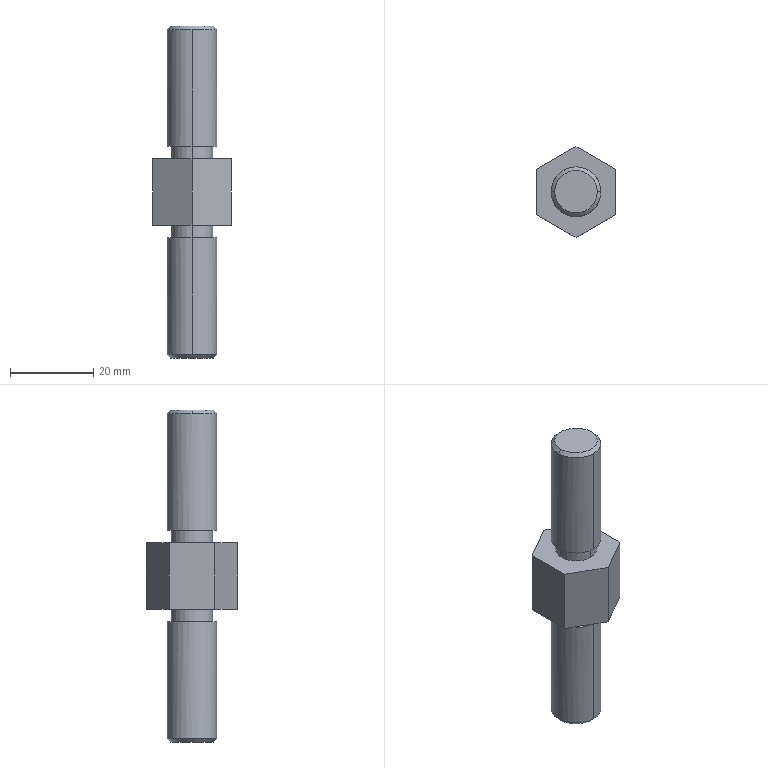Part | NX | 1 solid | 24 faces | box 19 x 21.939 x 80 mm | volume 12006 mm3 | plane 12 | cylinder 8 | cone 4 | commonest cylinder face diameters 10 x4 12 x4
STEP:
#1=CARTESIAN_POINT('',(0.,6.,11.));
#2=VERTEX_POINT('',#1);
#3=CARTESIAN_POINT('',(0.,-6.,11.));
#4=VERTEX_POINT('',#3);
#5=CARTESIAN_POINT('',(0.,0.,11.));
#6=DIRECTION('',(0.,0.,1.));
#7=DIRECTION('',(0.,-1.,0.));
#8=AXIS2_PLACEMENT_3D('',#5,#6,#7);
#9=CIRCLE('',#8,6.);
#10=EDGE_CURVE('',#2,#4,#9,.T.);
#11=ORIENTED_EDGE('',*,*,#10,.T.);
#12=CARTESIAN_POINT('',(0.,-6.,39.125));
#13=VERTEX_POINT('',#12);
#14=CARTESIAN_POINT('',(0.,-6.,5.));
#15=DIRECTION('',(0.,0.,1.));
#16=VECTOR('',#15,1000.);
#17=LINE('',#14,#16);
#18=EDGE_CURVE('',#13,#4,#17,.F.);
#19=ORIENTED_EDGE('',*,*,#18,.F.);
#20=CARTESIAN_POINT('',(-6.,0.,39.125));
#21=VERTEX_POINT('',#20);
#22=CARTESIAN_POINT('',(0.,0.,39.125));
#23=DIRECTION('',(0.,0.,-1.));
#24=DIRECTION('',(-1.,0.,0.));
#25=AXIS2_PLACEMENT_3D('',#22,#23,#24);
#26=CIRCLE('',#25,6.);
#27=EDGE_CURVE('',#13,#21,#26,.T.);
#28=ORIENTED_EDGE('',*,*,#27,.T.);
#29=CARTESIAN_POINT('',(0.,6.,39.125));
#30=VERTEX_POINT('',#29);
#31=CARTESIAN_POINT('',(0.,0.,39.125));
#32=DIRECTION('',(0.,0.,-1.));
#33=DIRECTION('',(-1.,0.,0.));
#34=AXIS2_PLACEMENT_3D('',#31,#32,#33);
#35=CIRCLE('',#34,6.);
#36=EDGE_CURVE('',#21,#30,#35,.T.);
#37=ORIENTED_EDGE('',*,*,#36,.T.);
#38=CARTESIAN_POINT('',(0.,6.,5.));
#39=DIRECTION('',(0.,0.,1.));
#40=VECTOR('',#39,1000.);
#41=LINE('',#38,#40);
#42=EDGE_CURVE('',#30,#2,#41,.F.);
#43=ORIENTED_EDGE('',*,*,#42,.T.);
#44=EDGE_LOOP('',(#11,#19,#28,#37,#43));
#45=FACE_BOUND('',#44,.T.);
#46=CARTESIAN_POINT('',(0.,0.,5.));
#47=DIRECTION('',(0.,0.,1.));
#48=DIRECTION('',(0.,-1.,0.));
#49=AXIS2_PLACEMENT_3D('',#46,#47,#48);
#50=CYLINDRICAL_SURFACE('',#49,6.);
#51=ADVANCED_FACE('',(#45),#50,.T.);
#52=CARTESIAN_POINT('',(5.125,0.,40.));
#53=VERTEX_POINT('',#52);
#54=CARTESIAN_POINT('',(-5.125,0.,40.));
#55=VERTEX_POINT('',#54);
#56=CARTESIAN_POINT('',(0.,0.,40.));
#57=DIRECTION('',(0.,0.,-1.));
#58=DIRECTION('',(-1.,0.,0.));
#59=AXIS2_PLACEMENT_3D('',#56,#57,#58);
#60=CIRCLE('',#59,5.125);
#61=EDGE_CURVE('',#53,#55,#60,.T.);
#62=ORIENTED_EDGE('',*,*,#61,.F.);
#63=CARTESIAN_POINT('',(0.,0.,40.));
#64=DIRECTION('',(0.,0.,-1.));
#65=DIRECTION('',(-1.,0.,0.));
#66=AXIS2_PLACEMENT_3D('',#63,#64,#65);
#67=CIRCLE('',#66,5.125);
#68=EDGE_CURVE('',#55,#53,#67,.T.);
#69=ORIENTED_EDGE('',*,*,#68,.F.);
#70=EDGE_LOOP('',(#62,#69));
#71=FACE_BOUND('',#70,.T.);
#72=CARTESIAN_POINT('',(-4.214,5.931,40.));
#73=DIRECTION('',(0.,0.,1.));
#74=DIRECTION('',(1.,0.,0.));
#75=AXIS2_PLACEMENT_3D('',#72,#73,#74);
#76=PLANE('',#75);
#77=ADVANCED_FACE('',(#71),#76,.T.);
#78=CARTESIAN_POINT('',(0.,6.,-11.));
#79=VERTEX_POINT('',#78);
#80=CARTESIAN_POINT('',(0.,-6.,-11.));
#81=VERTEX_POINT('',#80);
#82=CARTESIAN_POINT('',(0.,0.,-11.));
#83=DIRECTION('',(0.,0.,-1.));
#84=DIRECTION('',(0.,-1.,0.));
#85=AXIS2_PLACEMENT_3D('',#82,#83,#84);
#86=CIRCLE('',#85,6.);
#87=EDGE_CURVE('',#79,#81,#86,.T.);
#88=ORIENTED_EDGE('',*,*,#87,.F.);
#89=CARTESIAN_POINT('',(0.,0.,-11.));
#90=DIRECTION('',(0.,0.,-1.));
#91=DIRECTION('',(0.,-1.,0.));
#92=AXIS2_PLACEMENT_3D('',#89,#90,#91);
#93=CIRCLE('',#92,6.);
#94=EDGE_CURVE('',#81,#79,#93,.T.);
#95=ORIENTED_EDGE('',*,*,#94,.F.);
#96=EDGE_LOOP('',(#88,#95));
#97=FACE_BOUND('',#96,.T.);
#98=CARTESIAN_POINT('',(0.,-5.,-11.));
#99=VERTEX_POINT('',#98);
#100=CARTESIAN_POINT('',(0.,5.,-11.));
#101=VERTEX_POINT('',#100);
#102=CARTESIAN_POINT('',(0.,0.,-11.));
#103=DIRECTION('',(0.,0.,-1.));
#104=DIRECTION('',(0.,1.,0.));
#105=AXIS2_PLACEMENT_3D('',#102,#103,#104);
#106=CIRCLE('',#105,5.);
#107=EDGE_CURVE('',#99,#101,#106,.T.);
#108=ORIENTED_EDGE('',*,*,#107,.T.);
#109=CARTESIAN_POINT('',(0.,0.,-11.));
#110=DIRECTION('',(0.,0.,-1.));
#111=DIRECTION('',(0.,1.,0.));
#112=AXIS2_PLACEMENT_3D('',#109,#110,#111);
#113=CIRCLE('',#112,5.);
#114=EDGE_CURVE('',#101,#99,#113,.T.);
#115=ORIENTED_EDGE('',*,*,#114,.T.);
#116=EDGE_LOOP('',(#108,#115));
#117=FACE_BOUND('',#116,.T.);
#118=CARTESIAN_POINT('',(-2.472,7.007,-11.));
#119=DIRECTION('',(0.,0.,-1.));
#120=DIRECTION('',(0.,-1.,0.));
#121=AXIS2_PLACEMENT_3D('',#118,#119,#120);
#122=PLANE('',#121);
#123=ADVANCED_FACE('',(#97,#117),#122,.F.);
#124=CARTESIAN_POINT('',(-9.5,5.485,8.));
#125=VERTEX_POINT('',#124);
#126=CARTESIAN_POINT('',(-9.5,5.485,-8.));
#127=VERTEX_POINT('',#126);
#128=CARTESIAN_POINT('',(-9.5,5.485,0.));
#129=DIRECTION('',(0.,0.,-1.));
#130=VECTOR('',#129,1000.);
#131=LINE('',#128,#130);
#132=EDGE_CURVE('',#125,#127,#131,.T.);
#133=ORIENTED_EDGE('',*,*,#132,.F.);
#134=CARTESIAN_POINT('',(0.,10.97,8.));
#135=VERTEX_POINT('',#134);
#136=CARTESIAN_POINT('',(0.,10.97,8.));
#137=DIRECTION('',(0.866,0.5,0.));
#138=VECTOR('',#137,1000.);
#139=LINE('',#136,#138);
#140=EDGE_CURVE('',#125,#135,#139,.T.);
#141=ORIENTED_EDGE('',*,*,#140,.T.);
#142=CARTESIAN_POINT('',(0.,10.97,-8.));
#143=VERTEX_POINT('',#142);
#144=CARTESIAN_POINT('',(0.,10.97,0.));
#145=DIRECTION('',(0.,0.,1.));
#146=VECTOR('',#145,1000.);
#147=LINE('',#144,#146);
#148=EDGE_CURVE('',#143,#135,#147,.T.);
#149=ORIENTED_EDGE('',*,*,#148,.F.);
#150=CARTESIAN_POINT('',(0.,10.97,-8.));
#151=DIRECTION('',(0.866,0.5,0.));
#152=VECTOR('',#151,1000.);
#153=LINE('',#150,#152);
#154=EDGE_CURVE('',#127,#143,#153,.T.);
#155=ORIENTED_EDGE('',*,*,#154,.F.);
#156=EDGE_LOOP('',(#133,#141,#149,#155));
#157=FACE_BOUND('',#156,.T.);
#158=CARTESIAN_POINT('',(-9.5,5.485,0.));
#159=DIRECTION('',(-0.5,0.866,0.));
#160=DIRECTION('',(0.,0.,1.));
#161=AXIS2_PLACEMENT_3D('',#158,#159,#160);
#162=PLANE('',#161);
#163=ADVANCED_FACE('',(#157),#162,.T.);
#164=CARTESIAN_POINT('',(9.5,5.485,8.));
#165=VERTEX_POINT('',#164);
#166=CARTESIAN_POINT('',(9.5,-5.485,8.));
#167=VERTEX_POINT('',#166);
#168=CARTESIAN_POINT('',(9.5,0.,8.));
#169=DIRECTION('',(0.,-1.,0.));
#170=VECTOR('',#169,1000.);
#171=LINE('',#168,#170);
#172=EDGE_CURVE('',#165,#167,#171,.T.);
#173=ORIENTED_EDGE('',*,*,#172,.F.);
#174=CARTESIAN_POINT('',(0.,10.97,8.));
#175=DIRECTION('',(0.866,-0.5,0.));
#176=VECTOR('',#175,1000.);
#177=LINE('',#174,#176);
#178=EDGE_CURVE('',#135,#165,#177,.T.);
#179=ORIENTED_EDGE('',*,*,#178,.F.);
#180=ORIENTED_EDGE('',*,*,#140,.F.);
#181=CARTESIAN_POINT('',(-9.5,-5.485,8.));
#182=VERTEX_POINT('',#181);
#183=CARTESIAN_POINT('',(-9.5,0.,8.));
#184=DIRECTION('',(0.,1.,0.));
#185=VECTOR('',#184,1000.);
#186=LINE('',#183,#185);
#187=EDGE_CURVE('',#182,#125,#186,.T.);
#188=ORIENTED_EDGE('',*,*,#187,.F.);
#189=CARTESIAN_POINT('',(0.,-10.97,8.));
#190=VERTEX_POINT('',#189);
#191=CARTESIAN_POINT('',(0.,-10.97,8.));
#192=DIRECTION('',(-0.866,0.5,0.));
#193=VECTOR('',#192,1000.);
#194=LINE('',#191,#193);
#195=EDGE_CURVE('',#190,#182,#194,.T.);
#196=ORIENTED_EDGE('',*,*,#195,.F.);
#197=CARTESIAN_POINT('',(0.,-10.97,8.));
#198=DIRECTION('',(-0.866,-0.5,0.));
#199=VECTOR('',#198,1000.);
#200=LINE('',#197,#199);
#201=EDGE_CURVE('',#167,#190,#200,.T.);
#202=ORIENTED_EDGE('',*,*,#201,.F.);
#203=EDGE_LOOP('',(#173,#179,#180,#188,#196,#202));
#204=FACE_BOUND('',#203,.T.);
#205=CARTESIAN_POINT('',(0.,-5.,8.));
#206=VERTEX_POINT('',#205);
#207=CARTESIAN_POINT('',(0.,5.,8.));
#208=VERTEX_POINT('',#207);
#209=CARTESIAN_POINT('',(0.,0.,8.));
#210=DIRECTION('',(0.,0.,-1.));
#211=DIRECTION('',(0.,1.,0.));
#212=AXIS2_PLACEMENT_3D('',#209,#210,#211);
#213=CIRCLE('',#212,5.);
#214=EDGE_CURVE('',#206,#208,#213,.T.);
#215=ORIENTED_EDGE('',*,*,#214,.T.);
#216=CARTESIAN_POINT('',(0.,0.,8.));
#217=DIRECTION('',(0.,0.,-1.));
#218=DIRECTION('',(0.,1.,0.));
#219=AXIS2_PLACEMENT_3D('',#216,#217,#218);
#220=CIRCLE('',#219,5.);
#221=EDGE_CURVE('',#208,#206,#220,.T.);
#222=ORIENTED_EDGE('',*,*,#221,.T.);
#223=EDGE_LOOP('',(#215,#222));
#224=FACE_BOUND('',#223,.T.);
#225=CARTESIAN_POINT('',(-2.472,7.007,8.));
#226=DIRECTION('',(0.,0.,-1.));
#227=DIRECTION('',(0.,-1.,0.));
#228=AXIS2_PLACEMENT_3D('',#225,#226,#227);
#229=PLANE('',#228);
#230=ADVANCED_FACE('',(#204,#224),#229,.F.);
#231=CARTESIAN_POINT('',(9.5,-5.485,-8.));
#232=VERTEX_POINT('',#231);
#233=CARTESIAN_POINT('',(0.,-10.97,-8.));
#234=VERTEX_POINT('',#233);
#235=CARTESIAN_POINT('',(0.,-10.97,-8.));
#236=DIRECTION('',(-0.866,-0.5,0.));
#237=VECTOR('',#236,1000.);
#238=LINE('',#235,#237);
#239=EDGE_CURVE('',#232,#234,#238,.T.);
#240=ORIENTED_EDGE('',*,*,#239,.F.);
#241=CARTESIAN_POINT('',(9.5,-5.485,0.));
#242=DIRECTION('',(0.,0.,-1.));
#243=VECTOR('',#242,1000.);
#244=LINE('',#241,#243);
#245=EDGE_CURVE('',#167,#232,#244,.T.);
#246=ORIENTED_EDGE('',*,*,#245,.F.);
#247=ORIENTED_EDGE('',*,*,#201,.T.);
#248=CARTESIAN_POINT('',(0.,-10.97,0.));
#249=DIRECTION('',(0.,0.,-1.));
#250=VECTOR('',#249,1000.);
#251=LINE('',#248,#250);
#252=EDGE_CURVE('',#190,#234,#251,.T.);
#253=ORIENTED_EDGE('',*,*,#252,.T.);
#254=EDGE_LOOP('',(#240,#246,#247,#253));
#255=FACE_BOUND('',#254,.T.);
#256=CARTESIAN_POINT('',(9.5,-5.485,0.));
#257=DIRECTION('',(0.5,-0.866,0.));
#258=DIRECTION('',(0.,0.,-1.));
#259=AXIS2_PLACEMENT_3D('',#256,#257,#258);
#260=PLANE('',#259);
#261=ADVANCED_FACE('',(#255),#260,.T.);
#262=ORIENTED_EDGE('',*,*,#252,.F.);
#263=ORIENTED_EDGE('',*,*,#195,.T.);
#264=CARTESIAN_POINT('',(-9.5,-5.485,-8.));
#265=VERTEX_POINT('',#264);
#266=CARTESIAN_POINT('',(-9.5,-5.485,0.));
#267=DIRECTION('',(0.,0.,-1.));
#268=VECTOR('',#267,1000.);
#269=LINE('',#266,#268);
#270=EDGE_CURVE('',#182,#265,#269,.T.);
#271=ORIENTED_EDGE('',*,*,#270,.T.);
#272=CARTESIAN_POINT('',(0.,-10.97,-8.));
#273=DIRECTION('',(-0.866,0.5,0.));
#274=VECTOR('',#273,1000.);
#275=LINE('',#272,#274);
#276=EDGE_CURVE('',#234,#265,#275,.T.);
#277=ORIENTED_EDGE('',*,*,#276,.F.);
#278=EDGE_LOOP('',(#262,#263,#271,#277));
#279=FACE_BOUND('',#278,.T.);
#280=CARTESIAN_POINT('',(0.,-10.97,0.));
#281=DIRECTION('',(-0.5,-0.866,0.));
#282=DIRECTION('',(-0.866,0.5,0.));
#283=AXIS2_PLACEMENT_3D('',#280,#281,#282);
#284=PLANE('',#283);
#285=ADVANCED_FACE('',(#279),#284,.T.);
#286=ORIENTED_EDGE('',*,*,#270,.F.);
#287=ORIENTED_EDGE('',*,*,#187,.T.);
#288=ORIENTED_EDGE('',*,*,#132,.T.);
#289=CARTESIAN_POINT('',(-9.5,0.,-8.));
#290=DIRECTION('',(0.,1.,0.));
#291=VECTOR('',#290,1000.);
#292=LINE('',#289,#291);
#293=EDGE_CURVE('',#265,#127,#292,.T.);
#294=ORIENTED_EDGE('',*,*,#293,.F.);
#295=EDGE_LOOP('',(#286,#287,#288,#294));
#296=FACE_BOUND('',#295,.T.);
#297=CARTESIAN_POINT('',(-9.5,-5.485,0.));
#298=DIRECTION('',(-1.,0.,0.));
#299=DIRECTION('',(0.,0.,1.));
#300=AXIS2_PLACEMENT_3D('',#297,#298,#299);
#301=PLANE('',#300);
#302=ADVANCED_FACE('',(#296),#301,.T.);
#303=ORIENTED_EDGE('',*,*,#148,.T.);
#304=ORIENTED_EDGE('',*,*,#178,.T.);
#305=CARTESIAN_POINT('',(9.5,5.485,-8.));
#306=VERTEX_POINT('',#305);
#307=CARTESIAN_POINT('',(9.5,5.485,0.));
#308=DIRECTION('',(0.,0.,-1.));
#309=VECTOR('',#308,1000.);
#310=LINE('',#307,#309);
#311=EDGE_CURVE('',#165,#306,#310,.T.);
#312=ORIENTED_EDGE('',*,*,#311,.T.);
#313=CARTESIAN_POINT('',(0.,10.97,-8.));
#314=DIRECTION('',(0.866,-0.5,0.));
#315=VECTOR('',#314,1000.);
#316=LINE('',#313,#315);
#317=EDGE_CURVE('',#143,#306,#316,.T.);
#318=ORIENTED_EDGE('',*,*,#317,.F.);
#319=EDGE_LOOP('',(#303,#304,#312,#318));
#320=FACE_BOUND('',#319,.T.);
#321=CARTESIAN_POINT('',(0.,10.97,0.));
#322=DIRECTION('',(0.5,0.866,0.));
#323=DIRECTION('',(0.,0.,-1.));
#324=AXIS2_PLACEMENT_3D('',#321,#322,#323);
#325=PLANE('',#324);
#326=ADVANCED_FACE('',(#320),#325,.T.);
#327=ORIENTED_EDGE('',*,*,#87,.T.);
#328=CARTESIAN_POINT('',(0.,-6.,-39.125));
#329=VERTEX_POINT('',#328);
#330=CARTESIAN_POINT('',(0.,-6.,-5.));
#331=DIRECTION('',(0.,0.,-1.));
#332=VECTOR('',#331,1000.);
#333=LINE('',#330,#332);
#334=EDGE_CURVE('',#329,#81,#333,.F.);
#335=ORIENTED_EDGE('',*,*,#334,.F.);
#336=CARTESIAN_POINT('',(6.,0.,-39.125));
#337=VERTEX_POINT('',#336);
#338=CARTESIAN_POINT('',(0.,0.,-39.125));
#339=DIRECTION('',(0.,0.,1.));
#340=DIRECTION('',(1.,0.,0.));
#341=AXIS2_PLACEMENT_3D('',#338,#339,#340);
#342=CIRCLE('',#341,6.);
#343=EDGE_CURVE('',#329,#337,#342,.T.);
#344=ORIENTED_EDGE('',*,*,#343,.T.);
#345=CARTESIAN_POINT('',(0.,6.,-39.125));
#346=VERTEX_POINT('',#345);
#347=CARTESIAN_POINT('',(0.,0.,-39.125));
#348=DIRECTION('',(0.,0.,1.));
#349=DIRECTION('',(1.,0.,0.));
#350=AXIS2_PLACEMENT_3D('',#347,#348,#349);
#351=CIRCLE('',#350,6.);
#352=EDGE_CURVE('',#337,#346,#351,.T.);
#353=ORIENTED_EDGE('',*,*,#352,.T.);
#354=CARTESIAN_POINT('',(0.,6.,-5.));
#355=DIRECTION('',(0.,0.,-1.));
#356=VECTOR('',#355,1000.);
#357=LINE('',#354,#356);
#358=EDGE_CURVE('',#346,#79,#357,.F.);
#359=ORIENTED_EDGE('',*,*,#358,.T.);
#360=EDGE_LOOP('',(#327,#335,#344,#353,#359));
#361=FACE_BOUND('',#360,.T.);
#362=CARTESIAN_POINT('',(0.,0.,-5.));
#363=DIRECTION('',(0.,0.,-1.));
#364=DIRECTION('',(0.,-1.,0.));
#365=AXIS2_PLACEMENT_3D('',#362,#363,#364);
#366=CYLINDRICAL_SURFACE('',#365,6.);
#367=ADVANCED_FACE('',(#361),#366,.T.);
#368=CARTESIAN_POINT('',(5.125,0.,-40.));
#369=VERTEX_POINT('',#368);
#370=CARTESIAN_POINT('',(-5.125,0.,-40.));
#371=VERTEX_POINT('',#370);
#372=CARTESIAN_POINT('',(0.,0.,-40.));
#373=DIRECTION('',(0.,0.,1.));
#374=DIRECTION('',(1.,0.,0.));
#375=AXIS2_PLACEMENT_3D('',#372,#373,#374);
#376=CIRCLE('',#375,5.125);
#377=EDGE_CURVE('',#369,#371,#376,.T.);
#378=ORIENTED_EDGE('',*,*,#377,.F.);
#379=CARTESIAN_POINT('',(0.,0.,-40.));
#380=DIRECTION('',(0.,0.,1.));
#381=DIRECTION('',(1.,0.,0.));
#382=AXIS2_PLACEMENT_3D('',#379,#380,#381);
#383=CIRCLE('',#382,5.125);
#384=EDGE_CURVE('',#371,#369,#383,.T.);
#385=ORIENTED_EDGE('',*,*,#384,.F.);
#386=EDGE_LOOP('',(#378,#385));
#387=FACE_BOUND('',#386,.T.);
#388=CARTESIAN_POINT('',(0.,4.799,-40.));
#389=DIRECTION('',(0.,0.,-1.));
#390=DIRECTION('',(0.,-1.,0.));
#391=AXIS2_PLACEMENT_3D('',#388,#389,#390);
#392=PLANE('',#391);
#393=ADVANCED_FACE('',(#387),#392,.T.);
#394=ORIENTED_EDGE('',*,*,#311,.F.);
#395=ORIENTED_EDGE('',*,*,#172,.T.);
#396=ORIENTED_EDGE('',*,*,#245,.T.);
#397=CARTESIAN_POINT('',(9.5,0.,-8.));
#398=DIRECTION('',(0.,-1.,0.));
#399=VECTOR('',#398,1000.);
#400=LINE('',#397,#399);
#401=EDGE_CURVE('',#306,#232,#400,.T.);
#402=ORIENTED_EDGE('',*,*,#401,.F.);
#403=EDGE_LOOP('',(#394,#395,#396,#402));
#404=FACE_BOUND('',#403,.T.);
#405=CARTESIAN_POINT('',(9.5,5.485,0.));
#406=DIRECTION('',(1.,0.,0.));
#407=DIRECTION('',(0.,1.,0.));
#408=AXIS2_PLACEMENT_3D('',#405,#406,#407);
#409=PLANE('',#408);
#410=ADVANCED_FACE('',(#404),#409,.T.);
#411=ORIENTED_EDGE('',*,*,#214,.F.);
#412=CARTESIAN_POINT('',(0.,-5.,11.));
#413=VERTEX_POINT('',#412);
#414=CARTESIAN_POINT('',(0.,-5.,8.));
#415=DIRECTION('',(0.,0.,-1.));
#416=VECTOR('',#415,1000.);
#417=LINE('',#414,#416);
#418=EDGE_CURVE('',#413,#206,#417,.T.);
#419=ORIENTED_EDGE('',*,*,#418,.F.);
#420=CARTESIAN_POINT('',(0.,5.,11.));
#421=VERTEX_POINT('',#420);
#422=CARTESIAN_POINT('',(0.,0.,11.));
#423=DIRECTION('',(0.,0.,-1.));
#424=DIRECTION('',(0.,1.,0.));
#425=AXIS2_PLACEMENT_3D('',#422,#423,#424);
#426=CIRCLE('',#425,5.);
#427=EDGE_CURVE('',#413,#421,#426,.T.);
#428=ORIENTED_EDGE('',*,*,#427,.T.);
#429=CARTESIAN_POINT('',(0.,5.,8.));
#430=DIRECTION('',(0.,0.,-1.));
#431=VECTOR('',#430,1000.);
#432=LINE('',#429,#431);
#433=EDGE_CURVE('',#421,#208,#432,.T.);
#434=ORIENTED_EDGE('',*,*,#433,.T.);
#435=EDGE_LOOP('',(#411,#419,#428,#434));
#436=FACE_BOUND('',#435,.T.);
#437=CARTESIAN_POINT('',(0.,0.,8.));
#438=DIRECTION('',(0.,0.,-1.));
#439=DIRECTION('',(0.,1.,0.));
#440=AXIS2_PLACEMENT_3D('',#437,#438,#439);
#441=CYLINDRICAL_SURFACE('',#440,5.);
#442=ADVANCED_FACE('',(#436),#441,.T.);
#443=ORIENTED_EDGE('',*,*,#10,.F.);
#444=CARTESIAN_POINT('',(0.,0.,11.));
#445=DIRECTION('',(0.,0.,1.));
#446=DIRECTION('',(0.,-1.,0.));
#447=AXIS2_PLACEMENT_3D('',#444,#445,#446);
#448=CIRCLE('',#447,6.);
#449=EDGE_CURVE('',#4,#2,#448,.T.);
#450=ORIENTED_EDGE('',*,*,#449,.F.);
#451=EDGE_LOOP('',(#443,#450));
#452=FACE_BOUND('',#451,.T.);
#453=ORIENTED_EDGE('',*,*,#427,.F.);
#454=CARTESIAN_POINT('',(0.,0.,11.));
#455=DIRECTION('',(0.,0.,-1.));
#456=DIRECTION('',(0.,1.,0.));
#457=AXIS2_PLACEMENT_3D('',#454,#455,#456);
#458=CIRCLE('',#457,5.);
#459=EDGE_CURVE('',#421,#413,#458,.T.);
#460=ORIENTED_EDGE('',*,*,#459,.F.);
#461=EDGE_LOOP('',(#453,#460));
#462=FACE_BOUND('',#461,.T.);
#463=CARTESIAN_POINT('',(-2.472,7.007,11.));
#464=DIRECTION('',(0.,0.,-1.));
#465=DIRECTION('',(0.,-1.,0.));
#466=AXIS2_PLACEMENT_3D('',#463,#464,#465);
#467=PLANE('',#466);
#468=ADVANCED_FACE('',(#452,#462),#467,.T.);
#469=ORIENTED_EDGE('',*,*,#276,.T.);
#470=ORIENTED_EDGE('',*,*,#293,.T.);
#471=ORIENTED_EDGE('',*,*,#154,.T.);
#472=ORIENTED_EDGE('',*,*,#317,.T.);
#473=ORIENTED_EDGE('',*,*,#401,.T.);
#474=ORIENTED_EDGE('',*,*,#239,.T.);
#475=EDGE_LOOP('',(#469,#470,#471,#472,#473,#474));
#476=FACE_BOUND('',#475,.T.);
#477=CARTESIAN_POINT('',(0.,-5.,-8.));
#478=VERTEX_POINT('',#477);
#479=CARTESIAN_POINT('',(0.,5.,-8.));
#480=VERTEX_POINT('',#479);
#481=CARTESIAN_POINT('',(0.,0.,-8.));
#482=DIRECTION('',(0.,0.,-1.));
#483=DIRECTION('',(0.,1.,0.));
#484=AXIS2_PLACEMENT_3D('',#481,#482,#483);
#485=CIRCLE('',#484,5.);
#486=EDGE_CURVE('',#478,#480,#485,.T.);
#487=ORIENTED_EDGE('',*,*,#486,.F.);
#488=CARTESIAN_POINT('',(0.,0.,-8.));
#489=DIRECTION('',(0.,0.,-1.));
#490=DIRECTION('',(0.,1.,0.));
#491=AXIS2_PLACEMENT_3D('',#488,#489,#490);
#492=CIRCLE('',#491,5.);
#493=EDGE_CURVE('',#480,#478,#492,.T.);
#494=ORIENTED_EDGE('',*,*,#493,.F.);
#495=EDGE_LOOP('',(#487,#494));
#496=FACE_BOUND('',#495,.T.);
#497=CARTESIAN_POINT('',(-2.472,7.007,-8.));
#498=DIRECTION('',(0.,0.,-1.));
#499=DIRECTION('',(0.,-1.,0.));
#500=AXIS2_PLACEMENT_3D('',#497,#498,#499);
#501=PLANE('',#500);
#502=ADVANCED_FACE('',(#476,#496),#501,.T.);
#503=ORIENTED_EDGE('',*,*,#486,.T.);
#504=CARTESIAN_POINT('',(0.,5.,-8.));
#505=DIRECTION('',(0.,0.,-1.));
#506=VECTOR('',#505,1000.);
#507=LINE('',#504,#506);
#508=EDGE_CURVE('',#480,#101,#507,.T.);
#509=ORIENTED_EDGE('',*,*,#508,.T.);
#510=ORIENTED_EDGE('',*,*,#107,.F.);
#511=CARTESIAN_POINT('',(0.,-5.,-8.));
#512=DIRECTION('',(0.,0.,-1.));
#513=VECTOR('',#512,1000.);
#514=LINE('',#511,#513);
#515=EDGE_CURVE('',#478,#99,#514,.T.);
#516=ORIENTED_EDGE('',*,*,#515,.F.);
#517=EDGE_LOOP('',(#503,#509,#510,#516));
#518=FACE_BOUND('',#517,.T.);
#519=CARTESIAN_POINT('',(0.,0.,-8.));
#520=DIRECTION('',(0.,0.,-1.));
#521=DIRECTION('',(0.,1.,0.));
#522=AXIS2_PLACEMENT_3D('',#519,#520,#521);
#523=CYLINDRICAL_SURFACE('',#522,5.);
#524=ADVANCED_FACE('',(#518),#523,.T.);
#525=ORIENTED_EDGE('',*,*,#61,.T.);
#526=CARTESIAN_POINT('',(-5.125,0.,40.));
#527=DIRECTION('',(-0.7071,0.,-0.7071));
#528=VECTOR('',#527,1000.);
#529=LINE('',#526,#528);
#530=EDGE_CURVE('',#55,#21,#529,.T.);
#531=ORIENTED_EDGE('',*,*,#530,.T.);
#532=ORIENTED_EDGE('',*,*,#27,.F.);
#533=CARTESIAN_POINT('',(6.,0.,39.125));
#534=VERTEX_POINT('',#533);
#535=CARTESIAN_POINT('',(0.,0.,39.125));
#536=DIRECTION('',(0.,0.,-1.));
#537=DIRECTION('',(-1.,0.,0.));
#538=AXIS2_PLACEMENT_3D('',#535,#536,#537);
#539=CIRCLE('',#538,6.);
#540=EDGE_CURVE('',#534,#13,#539,.T.);
#541=ORIENTED_EDGE('',*,*,#540,.F.);
#542=CARTESIAN_POINT('',(5.125,0.,40.));
#543=DIRECTION('',(0.7071,0.,-0.7071));
#544=VECTOR('',#543,1000.);
#545=LINE('',#542,#544);
#546=EDGE_CURVE('',#53,#534,#545,.T.);
#547=ORIENTED_EDGE('',*,*,#546,.F.);
#548=EDGE_LOOP('',(#525,#531,#532,#541,#547));
#549=FACE_BOUND('',#548,.T.);
#550=CARTESIAN_POINT('',(0.,0.,40.));
#551=DIRECTION('',(0.,0.,-1.));
#552=DIRECTION('',(-1.,0.,0.));
#553=AXIS2_PLACEMENT_3D('',#550,#551,#552);
#554=CONICAL_SURFACE('',#553,5.125,0.7854);
#555=ADVANCED_FACE('',(#549),#554,.T.);
#556=ORIENTED_EDGE('',*,*,#377,.T.);
#557=CARTESIAN_POINT('',(-6.,0.,-39.125));
#558=VERTEX_POINT('',#557);
#559=CARTESIAN_POINT('',(-5.125,0.,-40.));
#560=DIRECTION('',(-0.7071,0.,0.7071));
#561=VECTOR('',#560,1000.);
#562=LINE('',#559,#561);
#563=EDGE_CURVE('',#371,#558,#562,.T.);
#564=ORIENTED_EDGE('',*,*,#563,.T.);
#565=CARTESIAN_POINT('',(0.,0.,-39.125));
#566=DIRECTION('',(0.,0.,1.));
#567=DIRECTION('',(1.,0.,0.));
#568=AXIS2_PLACEMENT_3D('',#565,#566,#567);
#569=CIRCLE('',#568,6.);
#570=EDGE_CURVE('',#346,#558,#569,.T.);
#571=ORIENTED_EDGE('',*,*,#570,.F.);
#572=ORIENTED_EDGE('',*,*,#352,.F.);
#573=CARTESIAN_POINT('',(5.125,0.,-40.));
#574=DIRECTION('',(0.7071,0.,0.7071));
#575=VECTOR('',#574,1000.);
#576=LINE('',#573,#575);
#577=EDGE_CURVE('',#369,#337,#576,.T.);
#578=ORIENTED_EDGE('',*,*,#577,.F.);
#579=EDGE_LOOP('',(#556,#564,#571,#572,#578));
#580=FACE_BOUND('',#579,.T.);
#581=CARTESIAN_POINT('',(0.,0.,-40.));
#582=DIRECTION('',(0.,0.,1.));
#583=DIRECTION('',(1.,0.,0.));
#584=AXIS2_PLACEMENT_3D('',#581,#582,#583);
#585=CONICAL_SURFACE('',#584,5.125,0.7854);
#586=ADVANCED_FACE('',(#580),#585,.T.);
#587=ORIENTED_EDGE('',*,*,#433,.F.);
#588=ORIENTED_EDGE('',*,*,#459,.T.);
#589=ORIENTED_EDGE('',*,*,#418,.T.);
#590=ORIENTED_EDGE('',*,*,#221,.F.);
#591=EDGE_LOOP('',(#587,#588,#589,#590));
#592=FACE_BOUND('',#591,.T.);
#593=CARTESIAN_POINT('',(0.,0.,8.));
#594=DIRECTION('',(0.,0.,-1.));
#595=DIRECTION('',(0.,1.,0.));
#596=AXIS2_PLACEMENT_3D('',#593,#594,#595);
#597=CYLINDRICAL_SURFACE('',#596,5.);
#598=ADVANCED_FACE('',(#592),#597,.T.);
#599=ORIENTED_EDGE('',*,*,#577,.T.);
#600=ORIENTED_EDGE('',*,*,#343,.F.);
#601=CARTESIAN_POINT('',(0.,0.,-39.125));
#602=DIRECTION('',(0.,0.,1.));
#603=DIRECTION('',(1.,0.,0.));
#604=AXIS2_PLACEMENT_3D('',#601,#602,#603);
#605=CIRCLE('',#604,6.);
#606=EDGE_CURVE('',#558,#329,#605,.T.);
#607=ORIENTED_EDGE('',*,*,#606,.F.);
#608=ORIENTED_EDGE('',*,*,#563,.F.);
#609=ORIENTED_EDGE('',*,*,#384,.T.);
#610=EDGE_LOOP('',(#599,#600,#607,#608,#609));
#611=FACE_BOUND('',#610,.T.);
#612=CARTESIAN_POINT('',(0.,0.,-40.));
#613=DIRECTION('',(0.,0.,1.));
#614=DIRECTION('',(1.,0.,0.));
#615=AXIS2_PLACEMENT_3D('',#612,#613,#614);
#616=CONICAL_SURFACE('',#615,5.125,0.7854);
#617=ADVANCED_FACE('',(#611),#616,.T.);
#618=ORIENTED_EDGE('',*,*,#540,.T.);
#619=ORIENTED_EDGE('',*,*,#18,.T.);
#620=ORIENTED_EDGE('',*,*,#449,.T.);
#621=ORIENTED_EDGE('',*,*,#42,.F.);
#622=CARTESIAN_POINT('',(0.,0.,39.125));
#623=DIRECTION('',(0.,0.,-1.));
#624=DIRECTION('',(-1.,0.,0.));
#625=AXIS2_PLACEMENT_3D('',#622,#623,#624);
#626=CIRCLE('',#625,6.);
#627=EDGE_CURVE('',#30,#534,#626,.T.);
#628=ORIENTED_EDGE('',*,*,#627,.T.);
#629=EDGE_LOOP('',(#618,#619,#620,#621,#628));
#630=FACE_BOUND('',#629,.T.);
#631=CARTESIAN_POINT('',(0.,0.,5.));
#632=DIRECTION('',(0.,0.,1.));
#633=DIRECTION('',(0.,-1.,0.));
#634=AXIS2_PLACEMENT_3D('',#631,#632,#633);
#635=CYLINDRICAL_SURFACE('',#634,6.);
#636=ADVANCED_FACE('',(#630),#635,.T.);
#637=ORIENTED_EDGE('',*,*,#570,.T.);
#638=ORIENTED_EDGE('',*,*,#606,.T.);
#639=ORIENTED_EDGE('',*,*,#334,.T.);
#640=ORIENTED_EDGE('',*,*,#94,.T.);
#641=ORIENTED_EDGE('',*,*,#358,.F.);
#642=EDGE_LOOP('',(#637,#638,#639,#640,#641));
#643=FACE_BOUND('',#642,.T.);
#644=CARTESIAN_POINT('',(0.,0.,-5.));
#645=DIRECTION('',(0.,0.,-1.));
#646=DIRECTION('',(0.,-1.,0.));
#647=AXIS2_PLACEMENT_3D('',#644,#645,#646);
#648=CYLINDRICAL_SURFACE('',#647,6.);
#649=ADVANCED_FACE('',(#643),#648,.T.);
#650=ORIENTED_EDGE('',*,*,#546,.T.);
#651=ORIENTED_EDGE('',*,*,#627,.F.);
#652=ORIENTED_EDGE('',*,*,#36,.F.);
#653=ORIENTED_EDGE('',*,*,#530,.F.);
#654=ORIENTED_EDGE('',*,*,#68,.T.);
#655=EDGE_LOOP('',(#650,#651,#652,#653,#654));
#656=FACE_BOUND('',#655,.T.);
#657=CARTESIAN_POINT('',(0.,0.,40.));
#658=DIRECTION('',(0.,0.,-1.));
#659=DIRECTION('',(-1.,0.,0.));
#660=AXIS2_PLACEMENT_3D('',#657,#658,#659);
#661=CONICAL_SURFACE('',#660,5.125,0.7854);
#662=ADVANCED_FACE('',(#656),#661,.T.);
#663=ORIENTED_EDGE('',*,*,#508,.F.);
#664=ORIENTED_EDGE('',*,*,#493,.T.);
#665=ORIENTED_EDGE('',*,*,#515,.T.);
#666=ORIENTED_EDGE('',*,*,#114,.F.);
#667=EDGE_LOOP('',(#663,#664,#665,#666));
#668=FACE_BOUND('',#667,.T.);
#669=CARTESIAN_POINT('',(0.,0.,-8.));
#670=DIRECTION('',(0.,0.,-1.));
#671=DIRECTION('',(0.,1.,0.));
#672=AXIS2_PLACEMENT_3D('',#669,#670,#671);
#673=CYLINDRICAL_SURFACE('',#672,5.);
#674=ADVANCED_FACE('',(#668),#673,.T.);
#675=CLOSED_SHELL('',(#51,#77,#123,#163,#230,#261,#285,#302,#326,#367,#393,#410,#442,#468,#502,#524,#555,#586,#598,#617,#636,#649,#662,#674));
#676=MANIFOLD_SOLID_BREP('',#675);
#677=(LENGTH_UNIT()NAMED_UNIT(*)SI_UNIT(.MILLI.,.METRE.));
#678=UNCERTAINTY_MEASURE_WITH_UNIT(LENGTH_MEASURE(0.00001),#677,'','');
#679=(NAMED_UNIT(*)PLANE_ANGLE_UNIT()SI_UNIT($,.RADIAN.));
#680=(NAMED_UNIT(*)SI_UNIT($,.STERADIAN.)SOLID_ANGLE_UNIT());
#681=(GEOMETRIC_REPRESENTATION_CONTEXT(3)GLOBAL_UNCERTAINTY_ASSIGNED_CONTEXT((#678))GLOBAL_UNIT_ASSIGNED_CONTEXT((#677,#679,#680))REPRESENTATION_CONTEXT('',''));
#682=ADVANCED_BREP_SHAPE_REPRESENTATION('',(#676),#681);